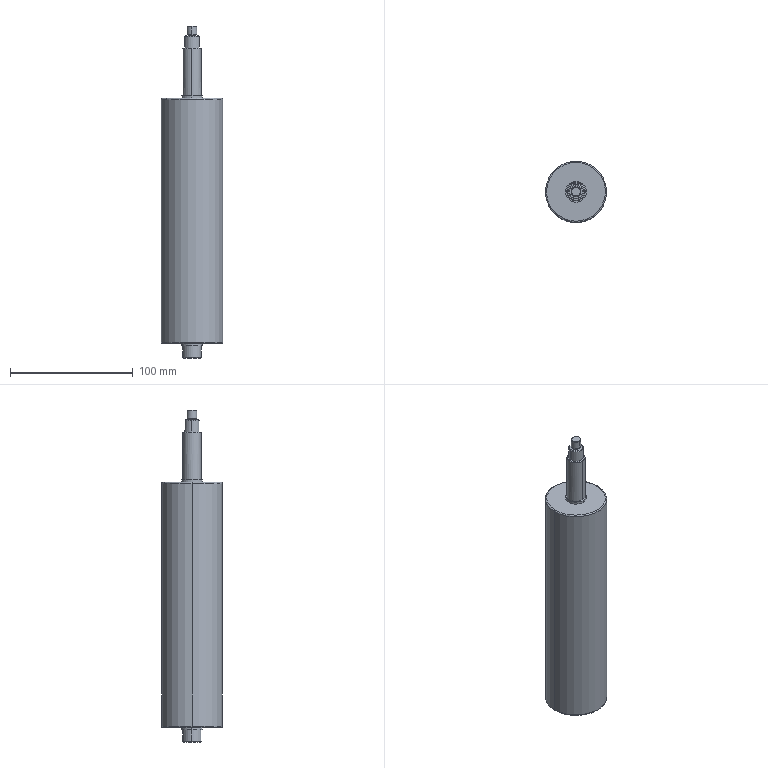Part | STEP file | 02-01 Driving mixing drum | 2 solids | 48 faces | box 50 x 50 x 271 mm | volume 629819 mm3 | cylinder 21 | plane 14 | cone 9 | spline 4 | commonest cylinder face diameters 15 x4 17 x4 12 x3 4 x2 6.4 x2 8 x2